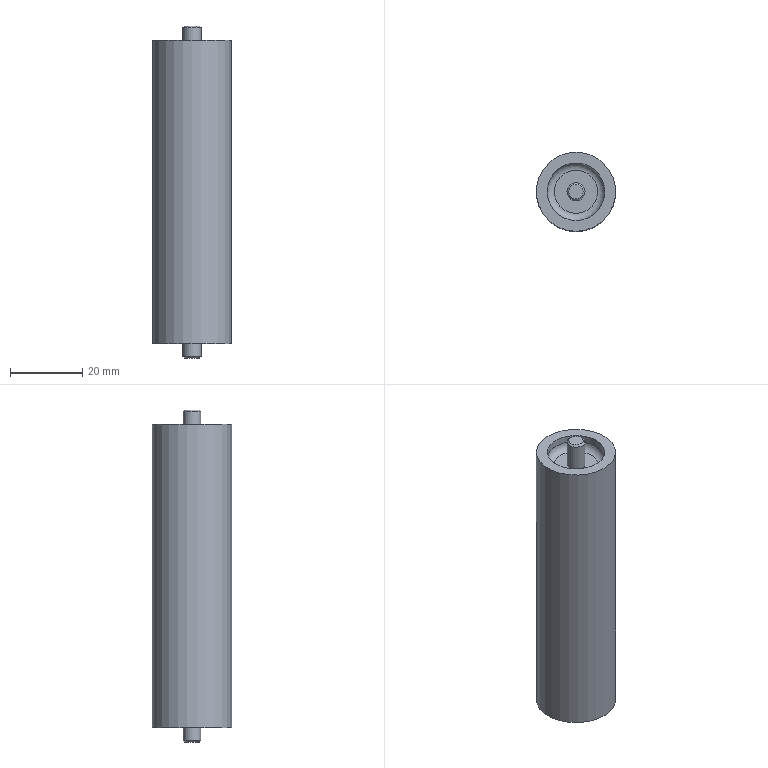Part | STEP file | Idler 2 | 1 solid | 15 faces | box 22 x 22 x 92.169 mm | volume 30779 mm3 | plane 6 | cylinder 5 | cone 2 | torus 2 | commonest cylinder face diameters 5 x2 16 x2 22 x1
STEP:
#1=CARTESIAN_POINT('',(0.07874,1.906,-1.814));
#2=VERTEX_POINT('',#1);
#3=CARTESIAN_POINT('',(0.,1.906,-1.814));
#4=DIRECTION('',(0.,0.,-1.));
#5=DIRECTION('',(-1.,0.,0.));
#6=AXIS2_PLACEMENT_3D('',#3,#4,#5);
#7=CIRCLE('',#6,0.07874);
#8=EDGE_CURVE('',#2,#2,#7,.T.);
#9=ORIENTED_EDGE('',*,*,#8,.F.);
#10=CARTESIAN_POINT('',(0.09843,1.906,-1.795));
#11=VERTEX_POINT('',#10);
#12=CARTESIAN_POINT('',(0.08858,1.906,-1.805));
#13=DIRECTION('',(0.7071,0.,0.7071));
#14=VECTOR('',#13,0.08858);
#15=LINE('',#12,#14);
#16=EDGE_CURVE('',#2,#11,#15,.T.);
#17=ORIENTED_EDGE('',*,*,#16,.T.);
#18=CARTESIAN_POINT('',(-0.09843,1.906,-1.795));
#19=VERTEX_POINT('',#18);
#20=CARTESIAN_POINT('',(0.,1.906,-1.795));
#21=DIRECTION('',(0.,0.,1.));
#22=DIRECTION('',(-1.,0.,0.));
#23=AXIS2_PLACEMENT_3D('',#20,#21,#22);
#24=CIRCLE('',#23,0.09843);
#25=EDGE_CURVE('',#19,#11,#24,.T.);
#26=ORIENTED_EDGE('',*,*,#25,.F.);
#27=CARTESIAN_POINT('',(0.,1.906,-1.795));
#28=DIRECTION('',(0.,0.,1.));
#29=DIRECTION('',(-1.,0.,0.));
#30=AXIS2_PLACEMENT_3D('',#27,#28,#29);
#31=CIRCLE('',#30,0.09843);
#32=EDGE_CURVE('',#11,#19,#31,.T.);
#33=ORIENTED_EDGE('',*,*,#32,.F.);
#34=ORIENTED_EDGE('',*,*,#16,.F.);
#35=EDGE_LOOP('',(#9,#17,#26,#33,#34));
#36=FACE_OUTER_BOUND('',#35,.T.);
#37=CARTESIAN_POINT('',(0.,1.906,-1.805));
#38=DIRECTION('',(0.,0.,1.));
#39=DIRECTION('',(-1.,0.,0.));
#40=AXIS2_PLACEMENT_3D('',#37,#38,#39);
#41=CONICAL_SURFACE('',#40,0.08858,0.7854);
#42=ADVANCED_FACE('',(#36),#41,.T.);
#43=ORIENTED_EDGE('',*,*,#32,.T.);
#44=CARTESIAN_POINT('',(-0.09843,1.906,-1.499));
#45=VERTEX_POINT('',#44);
#46=CARTESIAN_POINT('',(-0.09843,1.906,-1.499));
#47=DIRECTION('',(0.,0.,1.));
#48=VECTOR('',#47,0.09843);
#49=LINE('',#46,#48);
#50=EDGE_CURVE('',#19,#45,#49,.T.);
#51=ORIENTED_EDGE('',*,*,#50,.T.);
#52=CARTESIAN_POINT('',(0.,1.906,-1.499));
#53=DIRECTION('',(0.,0.,1.));
#54=DIRECTION('',(1.,0.,0.));
#55=AXIS2_PLACEMENT_3D('',#52,#53,#54);
#56=CIRCLE('',#55,0.09843);
#57=EDGE_CURVE('',#45,#45,#56,.T.);
#58=ORIENTED_EDGE('',*,*,#57,.F.);
#59=ORIENTED_EDGE('',*,*,#50,.F.);
#60=ORIENTED_EDGE('',*,*,#25,.T.);
#61=EDGE_LOOP('',(#43,#51,#58,#59,#60));
#62=FACE_OUTER_BOUND('',#61,.T.);
#63=CARTESIAN_POINT('',(0.,1.906,-1.499));
#64=DIRECTION('',(0.,0.,1.));
#65=DIRECTION('',(1.,0.,0.));
#66=AXIS2_PLACEMENT_3D('',#63,#64,#65);
#67=CYLINDRICAL_SURFACE('',#66,0.09843);
#68=ADVANCED_FACE('',(#62),#67,.T.);
#69=ORIENTED_EDGE('',*,*,#8,.T.);
#70=EDGE_LOOP('',(#69));
#71=FACE_OUTER_BOUND('',#70,.T.);
#72=CARTESIAN_POINT('',(0.,1.906,-1.814));
#73=DIRECTION('',(0.,0.,1.));
#74=DIRECTION('',(1.,0.,0.));
#75=AXIS2_PLACEMENT_3D('',#72,#73,#74);
#76=PLANE('',#75);
#77=ADVANCED_FACE('',(#71),#76,.F.);
#78=CARTESIAN_POINT('',(0.07874,1.906,1.814));
#79=VERTEX_POINT('',#78);
#80=CARTESIAN_POINT('',(0.,1.906,1.814));
#81=DIRECTION('',(0.,0.,-1.));
#82=DIRECTION('',(-1.,0.,0.));
#83=AXIS2_PLACEMENT_3D('',#80,#81,#82);
#84=CIRCLE('',#83,0.07874);
#85=EDGE_CURVE('',#79,#79,#84,.T.);
#86=ORIENTED_EDGE('',*,*,#85,.T.);
#87=CARTESIAN_POINT('',(0.09843,1.906,1.795));
#88=VERTEX_POINT('',#87);
#89=CARTESIAN_POINT('',(0.08858,1.906,1.805));
#90=DIRECTION('',(0.7071,0.,-0.7071));
#91=VECTOR('',#90,0.08858);
#92=LINE('',#89,#91);
#93=EDGE_CURVE('',#79,#88,#92,.T.);
#94=ORIENTED_EDGE('',*,*,#93,.T.);
#95=CARTESIAN_POINT('',(-0.09843,1.906,1.795));
#96=VERTEX_POINT('',#95);
#97=CARTESIAN_POINT('',(0.,1.906,1.795));
#98=DIRECTION('',(0.,0.,1.));
#99=DIRECTION('',(-1.,0.,0.));
#100=AXIS2_PLACEMENT_3D('',#97,#98,#99);
#101=CIRCLE('',#100,0.09843);
#102=EDGE_CURVE('',#88,#96,#101,.T.);
#103=ORIENTED_EDGE('',*,*,#102,.T.);
#104=CARTESIAN_POINT('',(0.,1.906,1.795));
#105=DIRECTION('',(0.,0.,1.));
#106=DIRECTION('',(-1.,0.,0.));
#107=AXIS2_PLACEMENT_3D('',#104,#105,#106);
#108=CIRCLE('',#107,0.09843);
#109=EDGE_CURVE('',#96,#88,#108,.T.);
#110=ORIENTED_EDGE('',*,*,#109,.T.);
#111=ORIENTED_EDGE('',*,*,#93,.F.);
#112=EDGE_LOOP('',(#86,#94,#103,#110,#111));
#113=FACE_OUTER_BOUND('',#112,.T.);
#114=CARTESIAN_POINT('',(0.,1.906,1.805));
#115=DIRECTION('',(0.,0.,-1.));
#116=DIRECTION('',(-1.,0.,0.));
#117=AXIS2_PLACEMENT_3D('',#114,#115,#116);
#118=CONICAL_SURFACE('',#117,0.08858,0.7854);
#119=ADVANCED_FACE('',(#113),#118,.T.);
#120=ORIENTED_EDGE('',*,*,#102,.F.);
#121=ORIENTED_EDGE('',*,*,#109,.F.);
#122=CARTESIAN_POINT('',(-0.09843,1.906,1.499));
#123=VERTEX_POINT('',#122);
#124=CARTESIAN_POINT('',(-0.09843,1.906,1.499));
#125=DIRECTION('',(0.,0.,-1.));
#126=VECTOR('',#125,0.09843);
#127=LINE('',#124,#126);
#128=EDGE_CURVE('',#96,#123,#127,.T.);
#129=ORIENTED_EDGE('',*,*,#128,.T.);
#130=CARTESIAN_POINT('',(0.,1.906,1.499));
#131=DIRECTION('',(0.,0.,-1.));
#132=DIRECTION('',(1.,0.,0.));
#133=AXIS2_PLACEMENT_3D('',#130,#131,#132);
#134=CIRCLE('',#133,0.09843);
#135=EDGE_CURVE('',#123,#123,#134,.T.);
#136=ORIENTED_EDGE('',*,*,#135,.F.);
#137=ORIENTED_EDGE('',*,*,#128,.F.);
#138=EDGE_LOOP('',(#120,#121,#129,#136,#137));
#139=FACE_OUTER_BOUND('',#138,.T.);
#140=CARTESIAN_POINT('',(0.,1.906,1.499));
#141=DIRECTION('',(0.,0.,1.));
#142=DIRECTION('',(1.,0.,0.));
#143=AXIS2_PLACEMENT_3D('',#140,#141,#142);
#144=CYLINDRICAL_SURFACE('',#143,0.09843);
#145=ADVANCED_FACE('',(#139),#144,.T.);
#146=ORIENTED_EDGE('',*,*,#85,.F.);
#147=EDGE_LOOP('',(#146));
#148=FACE_OUTER_BOUND('',#147,.T.);
#149=CARTESIAN_POINT('',(0.,1.906,1.814));
#150=DIRECTION('',(0.,0.,1.));
#151=DIRECTION('',(1.,0.,0.));
#152=AXIS2_PLACEMENT_3D('',#149,#150,#151);
#153=PLANE('',#152);
#154=ADVANCED_FACE('',(#148),#153,.T.);
#155=CARTESIAN_POINT('',(0.315,1.906,-1.578));
#156=VERTEX_POINT('',#155);
#157=CARTESIAN_POINT('',(-0.315,1.906,-1.578));
#158=VERTEX_POINT('',#157);
#159=CARTESIAN_POINT('',(0.,1.906,-1.578));
#160=DIRECTION('',(0.,0.,-1.));
#161=DIRECTION('',(-1.,0.,0.));
#162=AXIS2_PLACEMENT_3D('',#159,#160,#161);
#163=CIRCLE('',#162,0.315);
#164=EDGE_CURVE('',#156,#158,#163,.T.);
#165=ORIENTED_EDGE('',*,*,#164,.T.);
#166=CARTESIAN_POINT('',(0.,1.906,-1.578));
#167=DIRECTION('',(0.,0.,-1.));
#168=DIRECTION('',(-1.,0.,0.));
#169=AXIS2_PLACEMENT_3D('',#166,#167,#168);
#170=CIRCLE('',#169,0.315);
#171=EDGE_CURVE('',#158,#156,#170,.T.);
#172=ORIENTED_EDGE('',*,*,#171,.T.);
#173=CARTESIAN_POINT('',(0.2362,1.906,-1.499));
#174=VERTEX_POINT('',#173);
#175=CARTESIAN_POINT('',(0.2362,1.906,-1.578));
#176=DIRECTION('',(0.,-1.,0.));
#177=DIRECTION('',(1.,0.,0.));
#178=AXIS2_PLACEMENT_3D('',#175,#176,#177);
#179=CIRCLE('',#178,0.07874);
#180=EDGE_CURVE('',#156,#174,#179,.T.);
#181=ORIENTED_EDGE('',*,*,#180,.T.);
#182=CARTESIAN_POINT('',(0.,1.906,-1.499));
#183=DIRECTION('',(0.,0.,1.));
#184=DIRECTION('',(-1.,0.,0.));
#185=AXIS2_PLACEMENT_3D('',#182,#183,#184);
#186=CIRCLE('',#185,0.2362);
#187=EDGE_CURVE('',#174,#174,#186,.T.);
#188=ORIENTED_EDGE('',*,*,#187,.T.);
#189=ORIENTED_EDGE('',*,*,#180,.F.);
#190=EDGE_LOOP('',(#165,#172,#181,#188,#189));
#191=FACE_OUTER_BOUND('',#190,.T.);
#192=CARTESIAN_POINT('',(0.,1.906,-1.578));
#193=DIRECTION('',(0.,0.,1.));
#194=DIRECTION('',(-1.,0.,0.));
#195=AXIS2_PLACEMENT_3D('',#192,#193,#194);
#196=TOROIDAL_SURFACE('',#195,0.2362,0.07874);
#197=ADVANCED_FACE('',(#191),#196,.F.);
#198=CARTESIAN_POINT('',(-0.315,1.906,-1.657));
#199=VERTEX_POINT('',#198);
#200=CARTESIAN_POINT('',(0.,1.906,-1.657));
#201=DIRECTION('',(0.,0.,1.));
#202=DIRECTION('',(1.,0.,0.));
#203=AXIS2_PLACEMENT_3D('',#200,#201,#202);
#204=CIRCLE('',#203,0.315);
#205=EDGE_CURVE('',#199,#199,#204,.T.);
#206=ORIENTED_EDGE('',*,*,#205,.F.);
#207=CARTESIAN_POINT('',(-0.315,1.906,-1.657));
#208=DIRECTION('',(0.,0.,1.));
#209=VECTOR('',#208,0.315);
#210=LINE('',#207,#209);
#211=EDGE_CURVE('',#199,#158,#210,.T.);
#212=ORIENTED_EDGE('',*,*,#211,.T.);
#213=ORIENTED_EDGE('',*,*,#164,.F.);
#214=ORIENTED_EDGE('',*,*,#171,.F.);
#215=ORIENTED_EDGE('',*,*,#211,.F.);
#216=EDGE_LOOP('',(#206,#212,#213,#214,#215));
#217=FACE_OUTER_BOUND('',#216,.T.);
#218=CARTESIAN_POINT('',(0.,1.906,-1.657));
#219=DIRECTION('',(0.,0.,-1.));
#220=DIRECTION('',(1.,0.,0.));
#221=AXIS2_PLACEMENT_3D('',#218,#219,#220);
#222=CYLINDRICAL_SURFACE('',#221,0.315);
#223=ADVANCED_FACE('',(#217),#222,.F.);
#224=ORIENTED_EDGE('',*,*,#187,.F.);
#225=EDGE_LOOP('',(#224));
#226=FACE_OUTER_BOUND('',#225,.T.);
#227=ORIENTED_EDGE('',*,*,#57,.T.);
#228=EDGE_LOOP('',(#227));
#229=FACE_BOUND('',#228,.T.);
#230=CARTESIAN_POINT('',(0.,1.906,-1.499));
#231=DIRECTION('',(0.,0.,1.));
#232=DIRECTION('',(1.,0.,0.));
#233=AXIS2_PLACEMENT_3D('',#230,#231,#232);
#234=PLANE('',#233);
#235=ADVANCED_FACE('',(#226,#229),#234,.F.);
#236=CARTESIAN_POINT('',(0.2362,1.906,1.499));
#237=VERTEX_POINT('',#236);
#238=CARTESIAN_POINT('',(0.,1.906,1.499));
#239=DIRECTION('',(0.,0.,-1.));
#240=DIRECTION('',(-1.,0.,0.));
#241=AXIS2_PLACEMENT_3D('',#238,#239,#240);
#242=CIRCLE('',#241,0.2362);
#243=EDGE_CURVE('',#237,#237,#242,.T.);
#244=ORIENTED_EDGE('',*,*,#243,.T.);
#245=CARTESIAN_POINT('',(0.315,1.906,1.578));
#246=VERTEX_POINT('',#245);
#247=CARTESIAN_POINT('',(0.2362,1.906,1.578));
#248=DIRECTION('',(0.,-1.,0.));
#249=DIRECTION('',(1.,0.,0.));
#250=AXIS2_PLACEMENT_3D('',#247,#248,#249);
#251=CIRCLE('',#250,0.07874);
#252=EDGE_CURVE('',#237,#246,#251,.T.);
#253=ORIENTED_EDGE('',*,*,#252,.T.);
#254=CARTESIAN_POINT('',(-0.315,1.906,1.578));
#255=VERTEX_POINT('',#254);
#256=CARTESIAN_POINT('',(0.,1.906,1.578));
#257=DIRECTION('',(0.,0.,1.));
#258=DIRECTION('',(-1.,0.,0.));
#259=AXIS2_PLACEMENT_3D('',#256,#257,#258);
#260=CIRCLE('',#259,0.315);
#261=EDGE_CURVE('',#246,#255,#260,.T.);
#262=ORIENTED_EDGE('',*,*,#261,.T.);
#263=CARTESIAN_POINT('',(0.,1.906,1.578));
#264=DIRECTION('',(0.,0.,1.));
#265=DIRECTION('',(-1.,0.,0.));
#266=AXIS2_PLACEMENT_3D('',#263,#264,#265);
#267=CIRCLE('',#266,0.315);
#268=EDGE_CURVE('',#255,#246,#267,.T.);
#269=ORIENTED_EDGE('',*,*,#268,.T.);
#270=ORIENTED_EDGE('',*,*,#252,.F.);
#271=EDGE_LOOP('',(#244,#253,#262,#269,#270));
#272=FACE_OUTER_BOUND('',#271,.T.);
#273=CARTESIAN_POINT('',(0.,1.906,1.578));
#274=DIRECTION('',(0.,0.,-1.));
#275=DIRECTION('',(-1.,0.,0.));
#276=AXIS2_PLACEMENT_3D('',#273,#274,#275);
#277=TOROIDAL_SURFACE('',#276,0.2362,0.07874);
#278=ADVANCED_FACE('',(#272),#277,.F.);
#279=CARTESIAN_POINT('',(-0.315,1.906,1.657));
#280=VERTEX_POINT('',#279);
#281=CARTESIAN_POINT('',(0.,1.906,1.657));
#282=DIRECTION('',(0.,0.,-1.));
#283=DIRECTION('',(1.,0.,0.));
#284=AXIS2_PLACEMENT_3D('',#281,#282,#283);
#285=CIRCLE('',#284,0.315);
#286=EDGE_CURVE('',#280,#280,#285,.T.);
#287=ORIENTED_EDGE('',*,*,#286,.F.);
#288=CARTESIAN_POINT('',(-0.315,1.906,1.657));
#289=DIRECTION('',(0.,0.,-1.));
#290=VECTOR('',#289,0.315);
#291=LINE('',#288,#290);
#292=EDGE_CURVE('',#280,#255,#291,.T.);
#293=ORIENTED_EDGE('',*,*,#292,.T.);
#294=ORIENTED_EDGE('',*,*,#261,.F.);
#295=ORIENTED_EDGE('',*,*,#268,.F.);
#296=ORIENTED_EDGE('',*,*,#292,.F.);
#297=EDGE_LOOP('',(#287,#293,#294,#295,#296));
#298=FACE_OUTER_BOUND('',#297,.T.);
#299=CARTESIAN_POINT('',(0.,1.906,1.657));
#300=DIRECTION('',(0.,0.,-1.));
#301=DIRECTION('',(1.,0.,0.));
#302=AXIS2_PLACEMENT_3D('',#299,#300,#301);
#303=CYLINDRICAL_SURFACE('',#302,0.315);
#304=ADVANCED_FACE('',(#298),#303,.F.);
#305=ORIENTED_EDGE('',*,*,#243,.F.);
#306=EDGE_LOOP('',(#305));
#307=FACE_OUTER_BOUND('',#306,.T.);
#308=ORIENTED_EDGE('',*,*,#135,.T.);
#309=EDGE_LOOP('',(#308));
#310=FACE_BOUND('',#309,.T.);
#311=CARTESIAN_POINT('',(0.,1.906,1.499));
#312=DIRECTION('',(0.,0.,1.));
#313=DIRECTION('',(1.,0.,0.));
#314=AXIS2_PLACEMENT_3D('',#311,#312,#313);
#315=PLANE('',#314);
#316=ADVANCED_FACE('',(#307,#310),#315,.T.);
#317=CARTESIAN_POINT('',(0.,1.473,-1.657));
#318=VERTEX_POINT('',#317);
#319=CARTESIAN_POINT('',(0.,1.906,-1.657));
#320=DIRECTION('',(0.,0.,-1.));
#321=DIRECTION('',(1.,0.,0.));
#322=AXIS2_PLACEMENT_3D('',#319,#320,#321);
#323=CIRCLE('',#322,0.4331);
#324=EDGE_CURVE('',#318,#318,#323,.T.);
#325=ORIENTED_EDGE('',*,*,#324,.T.);
#326=EDGE_LOOP('',(#325));
#327=FACE_OUTER_BOUND('',#326,.T.);
#328=ORIENTED_EDGE('',*,*,#205,.T.);
#329=EDGE_LOOP('',(#328));
#330=FACE_BOUND('',#329,.T.);
#331=CARTESIAN_POINT('',(0.,1.906,-1.657));
#332=DIRECTION('',(0.,0.,-1.));
#333=DIRECTION('',(-1.,0.,0.));
#334=AXIS2_PLACEMENT_3D('',#331,#332,#333);
#335=PLANE('',#334);
#336=ADVANCED_FACE('',(#327,#330),#335,.T.);
#337=CARTESIAN_POINT('',(0.,1.473,1.657));
#338=VERTEX_POINT('',#337);
#339=CARTESIAN_POINT('',(0.,1.906,1.657));
#340=DIRECTION('',(0.,0.,-1.));
#341=DIRECTION('',(1.,0.,0.));
#342=AXIS2_PLACEMENT_3D('',#339,#340,#341);
#343=CIRCLE('',#342,0.4331);
#344=EDGE_CURVE('',#338,#338,#343,.T.);
#345=ORIENTED_EDGE('',*,*,#344,.F.);
#346=EDGE_LOOP('',(#345));
#347=FACE_OUTER_BOUND('',#346,.T.);
#348=ORIENTED_EDGE('',*,*,#286,.T.);
#349=EDGE_LOOP('',(#348));
#350=FACE_BOUND('',#349,.T.);
#351=CARTESIAN_POINT('',(0.,2.339,1.657));
#352=DIRECTION('',(0.,0.,1.));
#353=DIRECTION('',(1.,0.,0.));
#354=AXIS2_PLACEMENT_3D('',#351,#352,#353);
#355=PLANE('',#354);
#356=ADVANCED_FACE('',(#347,#350),#355,.T.);
#357=ORIENTED_EDGE('',*,*,#324,.F.);
#358=CARTESIAN_POINT('',(0.,1.473,0.));
#359=DIRECTION('',(0.,0.,1.));
#360=VECTOR('',#359,0.4331);
#361=LINE('',#358,#360);
#362=EDGE_CURVE('',#318,#338,#361,.T.);
#363=ORIENTED_EDGE('',*,*,#362,.T.);
#364=ORIENTED_EDGE('',*,*,#344,.T.);
#365=ORIENTED_EDGE('',*,*,#362,.F.);
#366=EDGE_LOOP('',(#357,#363,#364,#365));
#367=FACE_OUTER_BOUND('',#366,.T.);
#368=CARTESIAN_POINT('',(0.,1.906,0.));
#369=DIRECTION('',(0.,0.,-1.));
#370=DIRECTION('',(0.,1.,0.));
#371=AXIS2_PLACEMENT_3D('',#368,#369,#370);
#372=CYLINDRICAL_SURFACE('',#371,0.4331);
#373=ADVANCED_FACE('',(#367),#372,.T.);
#374=CLOSED_SHELL('',(#42,#68,#77,#119,#145,#154,#197,#223,#235,#278,#304,#316,#336,#356,#373));
#375=MANIFOLD_SOLID_BREP('',#374);
#376=(LENGTH_UNIT()NAMED_UNIT(*)SI_UNIT(.MILLI.,.METRE.));
#377=LENGTH_MEASURE_WITH_UNIT(LENGTH_MEASURE(25.4),#376);
#378=DIMENSIONAL_EXPONENTS(1.,0.,0.,0.,0.,0.,0.);
#379=(CONVERSION_BASED_UNIT('inch',#377)LENGTH_UNIT()NAMED_UNIT(#378));
#380=UNCERTAINTY_MEASURE_WITH_UNIT(LENGTH_MEASURE(0.0003937),#379,'','');
#381=(NAMED_UNIT(*)PLANE_ANGLE_UNIT()SI_UNIT($,.RADIAN.));
#382=(NAMED_UNIT(*)SI_UNIT($,.STERADIAN.)SOLID_ANGLE_UNIT());
#383=(GEOMETRIC_REPRESENTATION_CONTEXT(3)GLOBAL_UNCERTAINTY_ASSIGNED_CONTEXT((#380))GLOBAL_UNIT_ASSIGNED_CONTEXT((#379,#381,#382))REPRESENTATION_CONTEXT('',''));
#384=ADVANCED_BREP_SHAPE_REPRESENTATION('',(#375),#383);